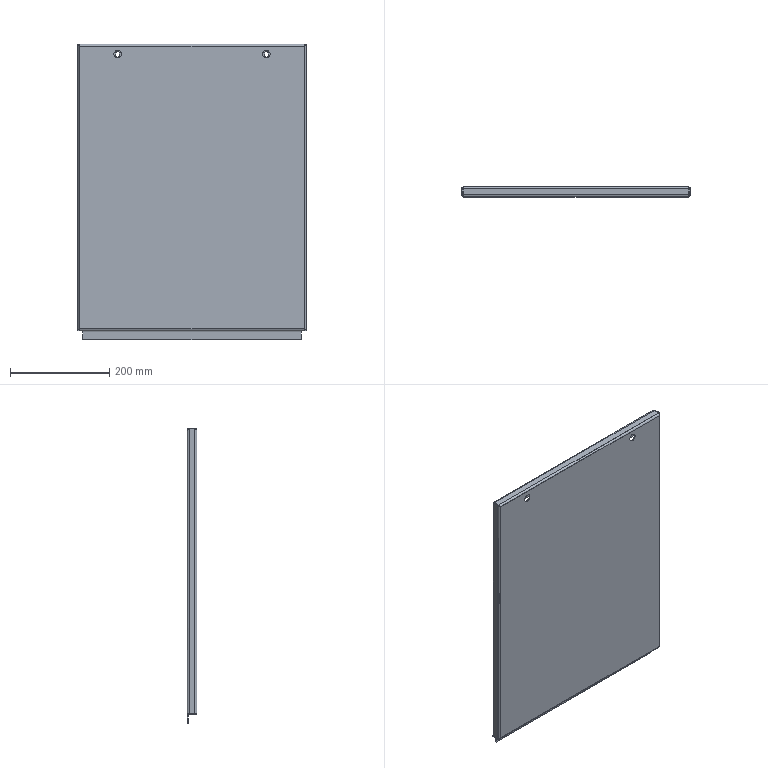Part | NX | features solid 2 | 1 solid | 104 faces | box 460 x 20 x 596 mm | volume 679401 mm3 | plane 70 | cylinder 26 | spline 8 | commonest cylinder face diameters 4 x8 8 x8 7 x6 15 x4